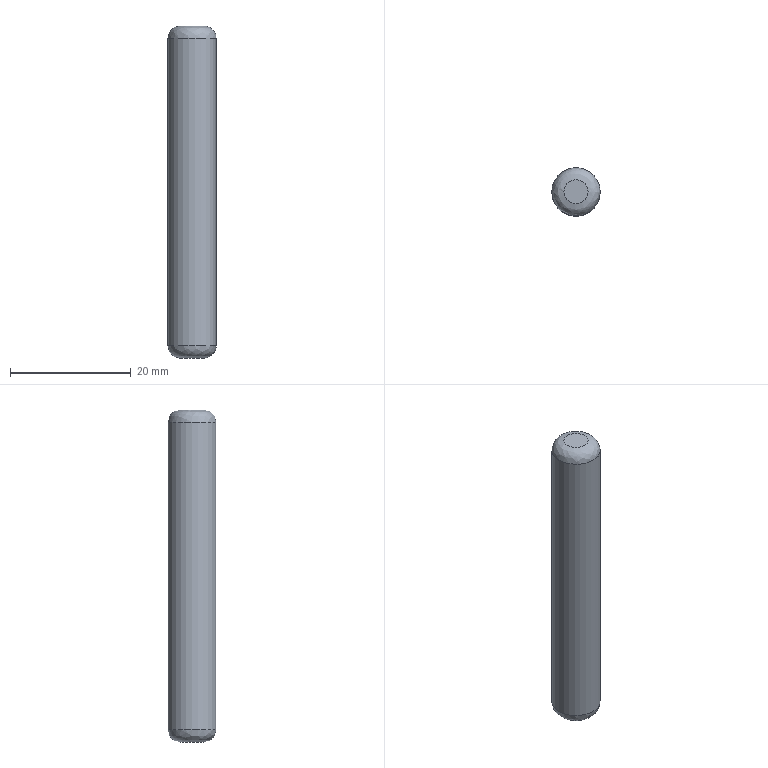Part | STEP file | 1 solid | 5 faces | box 8 x 8 x 55 mm | volume 2726 mm3 | plane 2 | spline 2 | cylinder 1 | commonest cylinder face diameters 8 x1
STEP:
#1=CARTESIAN_POINT('',(0.,0.,0.));
#2=DIRECTION('',(0.,0.,1.));
#3=DIRECTION('',(1.,0.,0.));
#4=AXIS2_PLACEMENT_3D('',#1,#2,#3);
#5=CARTESIAN_POINT('',(1516.247,357.48,61.619));
#6=VERTEX_POINT('',#5);
#7=CARTESIAN_POINT('',(1512.247,357.48,61.619));
#8=DIRECTION('',(0.,0.,-1.));
#9=DIRECTION('',(1.,0.,0.));
#10=AXIS2_PLACEMENT_3D('',#7,#8,#9);
#11=CIRCLE('',#10,4.);
#12=CARTESIAN_POINT('',(1512.247,357.48,8.619));
#13=DIRECTION('',(0.,0.,1.));
#14=DIRECTION('',(1.,0.,0.));
#15=AXIS2_PLACEMENT_3D('',#12,#13,#14);
#16=CYLINDRICAL_SURFACE('',#15,4.);
#17=CARTESIAN_POINT('',(6.283,53.));
#18=DIRECTION('',(-1.,0.));
#19=VECTOR('',#18,1.);
#20=LINE('',#17,#19);
#21=(GEOMETRIC_REPRESENTATION_CONTEXT(2)PARAMETRIC_REPRESENTATION_CONTEXT()REPRESENTATION_CONTEXT('',''));
#22=DEFINITIONAL_REPRESENTATION('',(#20),#21);
#23=PCURVE('',#16,#22);
#24=CARTESIAN_POINT('',(1508.247,357.48,61.619));
#25=CARTESIAN_POINT('',(1508.247,365.48,61.619));
#26=CARTESIAN_POINT('',(1516.247,365.48,61.619));
#27=CARTESIAN_POINT('',(1516.247,357.48,61.619));
#28=CARTESIAN_POINT('',(1516.247,349.48,61.619));
#29=CARTESIAN_POINT('',(1508.247,349.48,61.619));
#30=CARTESIAN_POINT('',(1508.247,357.48,61.619));
#31=CARTESIAN_POINT('',(1508.247,357.48,62.791));
#32=CARTESIAN_POINT('',(1508.247,365.48,62.791));
#33=CARTESIAN_POINT('',(1516.247,365.48,62.791));
#34=CARTESIAN_POINT('',(1516.247,357.48,62.791));
#35=CARTESIAN_POINT('',(1516.247,349.48,62.791));
#36=CARTESIAN_POINT('',(1508.247,349.48,62.791));
#37=CARTESIAN_POINT('',(1508.247,357.48,62.791));
#38=CARTESIAN_POINT('',(1509.076,357.48,63.619));
#39=CARTESIAN_POINT('',(1509.076,363.824,63.619));
#40=CARTESIAN_POINT('',(1515.419,363.824,63.619));
#41=CARTESIAN_POINT('',(1515.419,357.48,63.619));
#42=CARTESIAN_POINT('',(1515.419,351.137,63.619));
#43=CARTESIAN_POINT('',(1509.076,351.137,63.619));
#44=CARTESIAN_POINT('',(1509.076,357.48,63.619));
#45=CARTESIAN_POINT('',(1510.247,357.48,63.619));
#46=CARTESIAN_POINT('',(1510.247,361.48,63.619));
#47=CARTESIAN_POINT('',(1514.247,361.48,63.619));
#48=CARTESIAN_POINT('',(1514.247,357.48,63.619));
#49=CARTESIAN_POINT('',(1514.247,353.48,63.619));
#50=CARTESIAN_POINT('',(1510.247,353.48,63.619));
#51=CARTESIAN_POINT('',(1510.247,357.48,63.619));
#52=(BOUNDED_SURFACE()B_SPLINE_SURFACE(3,3,((#24,#25,#26,#27,#28,#29,#30),(#31,#32,#33,#34,#35,#36,#37),(#38,#39,#40,#41,#42,#43,#44),(#45,#46,#47,#48,#49,#50,#51)),.UNSPECIFIED.,.F.,.T.,.F.)B_SPLINE_SURFACE_WITH_KNOTS((4,4),(1,3,3,3,1),(0.,1.),(-0.5,0.,0.5,1.,1.5),.UNSPECIFIED.)GEOMETRIC_REPRESENTATION_ITEM()RATIONAL_B_SPLINE_SURFACE(((1.,0.3333,0.3333,1.,0.3333,0.3333,1.),(0.8047,0.2682,0.2682,0.8047,0.2682,0.2682,0.8047),(0.8047,0.2682,0.2682,0.8047,0.2682,0.2682,0.8047),(1.,0.3333,0.3333,1.,0.3333,0.3333,1.)))REPRESENTATION_ITEM('')SURFACE());
#53=CARTESIAN_POINT('',(0.,0.5));
#54=CARTESIAN_POINT('',(0.,0.5235));
#55=CARTESIAN_POINT('',(0.,0.5649));
#56=CARTESIAN_POINT('',(0.,0.6146));
#57=CARTESIAN_POINT('',(0.,0.6575));
#58=CARTESIAN_POINT('',(0.,0.696));
#59=CARTESIAN_POINT('',(0.,0.7322));
#60=CARTESIAN_POINT('',(0.,0.7678));
#61=CARTESIAN_POINT('',(0.,0.804));
#62=CARTESIAN_POINT('',(0.,0.8425));
#63=CARTESIAN_POINT('',(0.,0.8856));
#64=CARTESIAN_POINT('',(0.,0.9343));
#65=CARTESIAN_POINT('',(0.,1.));
#66=CARTESIAN_POINT('',(0.,1.066));
#67=CARTESIAN_POINT('',(0.,1.114));
#68=CARTESIAN_POINT('',(0.,1.158));
#69=CARTESIAN_POINT('',(0.,1.196));
#70=CARTESIAN_POINT('',(0.,1.232));
#71=CARTESIAN_POINT('',(0.,1.268));
#72=CARTESIAN_POINT('',(0.,1.304));
#73=CARTESIAN_POINT('',(0.,1.343));
#74=CARTESIAN_POINT('',(0.,1.385));
#75=CARTESIAN_POINT('',(0.,1.435));
#76=CARTESIAN_POINT('',(0.,1.476));
#77=CARTESIAN_POINT('',(0.,1.5));
#78=B_SPLINE_CURVE_WITH_KNOTS('',3,(#53,#54,#55,#56,#57,#58,#59,#60,#61,#62,#63,#64,#65,#66,#67,#68,#69,#70,#71,#72,#73,#74,#75,#76,#77),.UNSPECIFIED.,.F.,.F.,(4,1,1,1,1,1,1,1,1,1,1,1,1,1,1,1,1,1,1,1,1,1,4),(0.,0.2856,0.5712,0.8568,1.142,1.428,1.714,1.999,2.285,2.57,2.856,3.142,3.427,3.713,3.998,4.284,4.57,4.855,5.141,5.426,5.712,5.998,6.283),.QUASI_UNIFORM_KNOTS.);
#79=(GEOMETRIC_REPRESENTATION_CONTEXT(2)PARAMETRIC_REPRESENTATION_CONTEXT()REPRESENTATION_CONTEXT('',''));
#80=DEFINITIONAL_REPRESENTATION('',(#78),#79);
#81=PCURVE('',#52,#80);
#82=SURFACE_CURVE('',#11,(#23,#81),.PCURVE_S1.);
#83=EDGE_CURVE('',#6,#6,#82,.T.);
#84=ORIENTED_EDGE('',*,*,#83,.T.);
#85=CARTESIAN_POINT('',(1516.247,357.48,10.619));
#86=VERTEX_POINT('',#85);
#87=CARTESIAN_POINT('',(1516.247,357.48,10.619));
#88=CARTESIAN_POINT('',(1516.247,357.48,61.619));
#89=B_SPLINE_CURVE_WITH_KNOTS('',1,(#87,#88),.UNSPECIFIED.,.F.,.F.,(2,2),(2.,53.),.PIECEWISE_BEZIER_KNOTS.);
#90=CARTESIAN_POINT('',(0.,0.));
#91=DIRECTION('',(0.,1.));
#92=VECTOR('',#91,1.);
#93=LINE('',#90,#92);
#94=(GEOMETRIC_REPRESENTATION_CONTEXT(2)PARAMETRIC_REPRESENTATION_CONTEXT()REPRESENTATION_CONTEXT('',''));
#95=DEFINITIONAL_REPRESENTATION('',(#93),#94);
#96=PCURVE('',#16,#95);
#97=CARTESIAN_POINT('',(6.283,0.));
#98=DIRECTION('',(0.,1.));
#99=VECTOR('',#98,1.);
#100=LINE('',#97,#99);
#101=(GEOMETRIC_REPRESENTATION_CONTEXT(2)PARAMETRIC_REPRESENTATION_CONTEXT()REPRESENTATION_CONTEXT('',''));
#102=DEFINITIONAL_REPRESENTATION('',(#100),#101);
#103=PCURVE('',#16,#102);
#104=SEAM_CURVE('',#89,(#96,#103),.PCURVE_S1.);
#105=EDGE_CURVE('',#86,#6,#104,.T.);
#106=ORIENTED_EDGE('',*,*,#105,.F.);
#107=CARTESIAN_POINT('',(1512.247,357.48,10.619));
#108=DIRECTION('',(0.,0.,1.));
#109=DIRECTION('',(1.,0.,0.));
#110=AXIS2_PLACEMENT_3D('',#107,#108,#109);
#111=CIRCLE('',#110,4.);
#112=CARTESIAN_POINT('',(0.,2.));
#113=DIRECTION('',(1.,0.));
#114=VECTOR('',#113,1.);
#115=LINE('',#112,#114);
#116=(GEOMETRIC_REPRESENTATION_CONTEXT(2)PARAMETRIC_REPRESENTATION_CONTEXT()REPRESENTATION_CONTEXT('',''));
#117=DEFINITIONAL_REPRESENTATION('',(#115),#116);
#118=PCURVE('',#16,#117);
#119=CARTESIAN_POINT('',(1510.247,357.48,8.619));
#120=CARTESIAN_POINT('',(1510.247,361.48,8.619));
#121=CARTESIAN_POINT('',(1514.247,361.48,8.619));
#122=CARTESIAN_POINT('',(1514.247,357.48,8.619));
#123=CARTESIAN_POINT('',(1514.247,353.48,8.619));
#124=CARTESIAN_POINT('',(1510.247,353.48,8.619));
#125=CARTESIAN_POINT('',(1510.247,357.48,8.619));
#126=CARTESIAN_POINT('',(1509.076,357.48,8.619));
#127=CARTESIAN_POINT('',(1509.076,363.824,8.619));
#128=CARTESIAN_POINT('',(1515.419,363.824,8.619));
#129=CARTESIAN_POINT('',(1515.419,357.48,8.619));
#130=CARTESIAN_POINT('',(1515.419,351.137,8.619));
#131=CARTESIAN_POINT('',(1509.076,351.137,8.619));
#132=CARTESIAN_POINT('',(1509.076,357.48,8.619));
#133=CARTESIAN_POINT('',(1508.247,357.48,9.447));
#134=CARTESIAN_POINT('',(1508.247,365.48,9.447));
#135=CARTESIAN_POINT('',(1516.247,365.48,9.447));
#136=CARTESIAN_POINT('',(1516.247,357.48,9.447));
#137=CARTESIAN_POINT('',(1516.247,349.48,9.447));
#138=CARTESIAN_POINT('',(1508.247,349.48,9.447));
#139=CARTESIAN_POINT('',(1508.247,357.48,9.447));
#140=CARTESIAN_POINT('',(1508.247,357.48,10.619));
#141=CARTESIAN_POINT('',(1508.247,365.48,10.619));
#142=CARTESIAN_POINT('',(1516.247,365.48,10.619));
#143=CARTESIAN_POINT('',(1516.247,357.48,10.619));
#144=CARTESIAN_POINT('',(1516.247,349.48,10.619));
#145=CARTESIAN_POINT('',(1508.247,349.48,10.619));
#146=CARTESIAN_POINT('',(1508.247,357.48,10.619));
#147=(BOUNDED_SURFACE()B_SPLINE_SURFACE(3,3,((#119,#120,#121,#122,#123,#124,#125),(#126,#127,#128,#129,#130,#131,#132),(#133,#134,#135,#136,#137,#138,#139),(#140,#141,#142,#143,#144,#145,#146)),.UNSPECIFIED.,.F.,.T.,.F.)B_SPLINE_SURFACE_WITH_KNOTS((4,4),(1,3,3,3,1),(0.,1.),(-0.5,0.,0.5,1.,1.5),.UNSPECIFIED.)GEOMETRIC_REPRESENTATION_ITEM()RATIONAL_B_SPLINE_SURFACE(((1.,0.3333,0.3333,1.,0.3333,0.3333,1.),(0.8047,0.2682,0.2682,0.8047,0.2682,0.2682,0.8047),(0.8047,0.2682,0.2682,0.8047,0.2682,0.2682,0.8047),(1.,0.3333,0.3333,1.,0.3333,0.3333,1.)))REPRESENTATION_ITEM('')SURFACE());
#148=CARTESIAN_POINT('',(1.,1.5));
#149=CARTESIAN_POINT('',(1.,1.476));
#150=CARTESIAN_POINT('',(1.,1.435));
#151=CARTESIAN_POINT('',(1.,1.385));
#152=CARTESIAN_POINT('',(1.,1.343));
#153=CARTESIAN_POINT('',(1.,1.304));
#154=CARTESIAN_POINT('',(1.,1.268));
#155=CARTESIAN_POINT('',(1.,1.232));
#156=CARTESIAN_POINT('',(1.,1.196));
#157=CARTESIAN_POINT('',(1.,1.158));
#158=CARTESIAN_POINT('',(1.,1.114));
#159=CARTESIAN_POINT('',(1.,1.066));
#160=CARTESIAN_POINT('',(1.,1.));
#161=CARTESIAN_POINT('',(1.,0.9343));
#162=CARTESIAN_POINT('',(1.,0.8856));
#163=CARTESIAN_POINT('',(1.,0.8425));
#164=CARTESIAN_POINT('',(1.,0.804));
#165=CARTESIAN_POINT('',(1.,0.7678));
#166=CARTESIAN_POINT('',(1.,0.7322));
#167=CARTESIAN_POINT('',(1.,0.696));
#168=CARTESIAN_POINT('',(1.,0.6575));
#169=CARTESIAN_POINT('',(1.,0.6146));
#170=CARTESIAN_POINT('',(1.,0.5649));
#171=CARTESIAN_POINT('',(1.,0.5235));
#172=CARTESIAN_POINT('',(1.,0.5));
#173=B_SPLINE_CURVE_WITH_KNOTS('',3,(#148,#149,#150,#151,#152,#153,#154,#155,#156,#157,#158,#159,#160,#161,#162,#163,#164,#165,#166,#167,#168,#169,#170,#171,#172),.UNSPECIFIED.,.F.,.F.,(4,1,1,1,1,1,1,1,1,1,1,1,1,1,1,1,1,1,1,1,1,1,4),(0.,0.2856,0.5712,0.8568,1.142,1.428,1.714,1.999,2.285,2.57,2.856,3.142,3.427,3.713,3.998,4.284,4.57,4.855,5.141,5.426,5.712,5.998,6.283),.QUASI_UNIFORM_KNOTS.);
#174=(GEOMETRIC_REPRESENTATION_CONTEXT(2)PARAMETRIC_REPRESENTATION_CONTEXT()REPRESENTATION_CONTEXT('',''));
#175=DEFINITIONAL_REPRESENTATION('',(#173),#174);
#176=PCURVE('',#147,#175);
#177=SURFACE_CURVE('',#111,(#118,#176),.PCURVE_S1.);
#178=EDGE_CURVE('',#86,#86,#177,.T.);
#179=ORIENTED_EDGE('',*,*,#178,.T.);
#180=ORIENTED_EDGE('',*,*,#105,.T.);
#181=EDGE_LOOP('',(#84,#106,#179,#180));
#182=FACE_BOUND('',#181,.T.);
#183=ADVANCED_FACE('',(#182),#16,.T.);
#184=CARTESIAN_POINT('',(1514.247,357.48,8.619));
#185=VERTEX_POINT('',#184);
#186=CARTESIAN_POINT('',(1512.247,357.48,8.619));
#187=DIRECTION('',(0.,0.,-1.));
#188=DIRECTION('',(1.,0.,0.));
#189=AXIS2_PLACEMENT_3D('',#186,#187,#188);
#190=CIRCLE('',#189,2.);
#191=CARTESIAN_POINT('',(1512.247,357.48,8.619));
#192=DIRECTION('',(0.,0.,-1.));
#193=DIRECTION('',(-1.,0.,0.));
#194=AXIS2_PLACEMENT_3D('',#191,#192,#193);
#195=PLANE('',#194);
#196=CARTESIAN_POINT('',(0.,0.));
#197=DIRECTION('',(-1.,0.));
#198=AXIS2_PLACEMENT_2D('',#196,#197);
#199=CIRCLE('',#198,2.);
#200=(GEOMETRIC_REPRESENTATION_CONTEXT(2)PARAMETRIC_REPRESENTATION_CONTEXT()REPRESENTATION_CONTEXT('',''));
#201=DEFINITIONAL_REPRESENTATION('',(#199),#200);
#202=PCURVE('',#195,#201);
#203=CARTESIAN_POINT('',(0.,0.5));
#204=CARTESIAN_POINT('',(0.,0.5235));
#205=CARTESIAN_POINT('',(0.,0.5649));
#206=CARTESIAN_POINT('',(0.,0.6146));
#207=CARTESIAN_POINT('',(0.,0.6575));
#208=CARTESIAN_POINT('',(0.,0.696));
#209=CARTESIAN_POINT('',(0.,0.7322));
#210=CARTESIAN_POINT('',(0.,0.7678));
#211=CARTESIAN_POINT('',(0.,0.804));
#212=CARTESIAN_POINT('',(0.,0.8425));
#213=CARTESIAN_POINT('',(0.,0.8856));
#214=CARTESIAN_POINT('',(0.,0.9343));
#215=CARTESIAN_POINT('',(0.,1.));
#216=CARTESIAN_POINT('',(0.,1.066));
#217=CARTESIAN_POINT('',(0.,1.114));
#218=CARTESIAN_POINT('',(0.,1.158));
#219=CARTESIAN_POINT('',(0.,1.196));
#220=CARTESIAN_POINT('',(0.,1.232));
#221=CARTESIAN_POINT('',(0.,1.268));
#222=CARTESIAN_POINT('',(0.,1.304));
#223=CARTESIAN_POINT('',(0.,1.343));
#224=CARTESIAN_POINT('',(0.,1.385));
#225=CARTESIAN_POINT('',(0.,1.435));
#226=CARTESIAN_POINT('',(0.,1.476));
#227=CARTESIAN_POINT('',(0.,1.5));
#228=B_SPLINE_CURVE_WITH_KNOTS('',3,(#203,#204,#205,#206,#207,#208,#209,#210,#211,#212,#213,#214,#215,#216,#217,#218,#219,#220,#221,#222,#223,#224,#225,#226,#227),.UNSPECIFIED.,.F.,.F.,(4,1,1,1,1,1,1,1,1,1,1,1,1,1,1,1,1,1,1,1,1,1,4),(0.,0.2856,0.5712,0.8568,1.142,1.428,1.714,1.999,2.285,2.57,2.856,3.142,3.427,3.713,3.998,4.284,4.57,4.855,5.141,5.426,5.712,5.998,6.283),.QUASI_UNIFORM_KNOTS.);
#229=(GEOMETRIC_REPRESENTATION_CONTEXT(2)PARAMETRIC_REPRESENTATION_CONTEXT()REPRESENTATION_CONTEXT('',''));
#230=DEFINITIONAL_REPRESENTATION('',(#228),#229);
#231=PCURVE('',#147,#230);
#232=SURFACE_CURVE('',#190,(#202,#231),.PCURVE_S1.);
#233=EDGE_CURVE('',#185,#185,#232,.T.);
#234=ORIENTED_EDGE('',*,*,#233,.T.);
#235=EDGE_LOOP('',(#234));
#236=FACE_BOUND('',#235,.T.);
#237=ADVANCED_FACE('',(#236),#195,.T.);
#238=CARTESIAN_POINT('',(1514.247,357.48,63.619));
#239=VERTEX_POINT('',#238);
#240=CARTESIAN_POINT('',(1512.247,357.48,63.619));
#241=DIRECTION('',(0.,0.,1.));
#242=DIRECTION('',(1.,0.,0.));
#243=AXIS2_PLACEMENT_3D('',#240,#241,#242);
#244=CIRCLE('',#243,2.);
#245=CARTESIAN_POINT('',(1512.247,357.48,63.619));
#246=DIRECTION('',(0.,0.,-1.));
#247=DIRECTION('',(-1.,0.,0.));
#248=AXIS2_PLACEMENT_3D('',#245,#246,#247);
#249=PLANE('',#248);
#250=CARTESIAN_POINT('',(-2.,0.));
#251=CARTESIAN_POINT('',(-2.,3.464));
#252=CARTESIAN_POINT('',(1.,1.732));
#253=CARTESIAN_POINT('',(4.,0.));
#254=CARTESIAN_POINT('',(1.,-1.732));
#255=CARTESIAN_POINT('',(-2.,-3.464));
#256=CARTESIAN_POINT('',(-2.,0.));
#257=(BOUNDED_CURVE()B_SPLINE_CURVE(2,(#250,#251,#252,#253,#254,#255,#256),.UNSPECIFIED.,.T.,.F.)B_SPLINE_CURVE_WITH_KNOTS((1,2,2,2,2,1),(-2.094,0.,2.094,4.189,6.283,8.378),.UNSPECIFIED.)CURVE()GEOMETRIC_REPRESENTATION_ITEM()RATIONAL_B_SPLINE_CURVE((1.,0.5,1.,0.5,1.,0.5,1.))REPRESENTATION_ITEM(''));
#258=(GEOMETRIC_REPRESENTATION_CONTEXT(2)PARAMETRIC_REPRESENTATION_CONTEXT()REPRESENTATION_CONTEXT('',''));
#259=DEFINITIONAL_REPRESENTATION('',(#257),#258);
#260=PCURVE('',#249,#259);
#261=CARTESIAN_POINT('',(1.,1.5));
#262=CARTESIAN_POINT('',(1.,1.476));
#263=CARTESIAN_POINT('',(1.,1.435));
#264=CARTESIAN_POINT('',(1.,1.385));
#265=CARTESIAN_POINT('',(1.,1.343));
#266=CARTESIAN_POINT('',(1.,1.304));
#267=CARTESIAN_POINT('',(1.,1.268));
#268=CARTESIAN_POINT('',(1.,1.232));
#269=CARTESIAN_POINT('',(1.,1.196));
#270=CARTESIAN_POINT('',(1.,1.158));
#271=CARTESIAN_POINT('',(1.,1.114));
#272=CARTESIAN_POINT('',(1.,1.066));
#273=CARTESIAN_POINT('',(1.,1.));
#274=CARTESIAN_POINT('',(1.,0.9343));
#275=CARTESIAN_POINT('',(1.,0.8856));
#276=CARTESIAN_POINT('',(1.,0.8425));
#277=CARTESIAN_POINT('',(1.,0.804));
#278=CARTESIAN_POINT('',(1.,0.7678));
#279=CARTESIAN_POINT('',(1.,0.7322));
#280=CARTESIAN_POINT('',(1.,0.696));
#281=CARTESIAN_POINT('',(1.,0.6575));
#282=CARTESIAN_POINT('',(1.,0.6146));
#283=CARTESIAN_POINT('',(1.,0.5649));
#284=CARTESIAN_POINT('',(1.,0.5235));
#285=CARTESIAN_POINT('',(1.,0.5));
#286=B_SPLINE_CURVE_WITH_KNOTS('',3,(#261,#262,#263,#264,#265,#266,#267,#268,#269,#270,#271,#272,#273,#274,#275,#276,#277,#278,#279,#280,#281,#282,#283,#284,#285),.UNSPECIFIED.,.F.,.F.,(4,1,1,1,1,1,1,1,1,1,1,1,1,1,1,1,1,1,1,1,1,1,4),(0.,0.2856,0.5712,0.8568,1.142,1.428,1.714,1.999,2.285,2.57,2.856,3.142,3.427,3.713,3.998,4.284,4.57,4.855,5.141,5.426,5.712,5.998,6.283),.QUASI_UNIFORM_KNOTS.);
#287=(GEOMETRIC_REPRESENTATION_CONTEXT(2)PARAMETRIC_REPRESENTATION_CONTEXT()REPRESENTATION_CONTEXT('',''));
#288=DEFINITIONAL_REPRESENTATION('',(#286),#287);
#289=PCURVE('',#52,#288);
#290=SURFACE_CURVE('',#244,(#260,#289),.PCURVE_S1.);
#291=EDGE_CURVE('',#239,#239,#290,.T.);
#292=ORIENTED_EDGE('',*,*,#291,.T.);
#293=EDGE_LOOP('',(#292));
#294=FACE_BOUND('',#293,.T.);
#295=ADVANCED_FACE('',(#294),#249,.F.);
#296=ORIENTED_EDGE('',*,*,#291,.F.);
#297=CARTESIAN_POINT('',(1516.247,357.48,61.619));
#298=CARTESIAN_POINT('',(1516.247,357.48,62.791));
#299=CARTESIAN_POINT('',(1515.419,357.48,63.619));
#300=CARTESIAN_POINT('',(1514.247,357.48,63.619));
#301=(BOUNDED_CURVE()B_SPLINE_CURVE(3,(#297,#298,#299,#300),.UNSPECIFIED.,.F.,.F.)B_SPLINE_CURVE_WITH_KNOTS((4,4),(0.,1.),.PIECEWISE_BEZIER_KNOTS.)CURVE()GEOMETRIC_REPRESENTATION_ITEM()RATIONAL_B_SPLINE_CURVE((1.,0.8047,0.8047,1.))REPRESENTATION_ITEM(''));
#302=CARTESIAN_POINT('',(0.,1.5));
#303=DIRECTION('',(1.,0.));
#304=VECTOR('',#303,1.);
#305=LINE('',#302,#304);
#306=(GEOMETRIC_REPRESENTATION_CONTEXT(2)PARAMETRIC_REPRESENTATION_CONTEXT()REPRESENTATION_CONTEXT('',''));
#307=DEFINITIONAL_REPRESENTATION('',(#305),#306);
#308=PCURVE('',#52,#307);
#309=CARTESIAN_POINT('',(0.,0.5));
#310=DIRECTION('',(1.,0.));
#311=VECTOR('',#310,1.);
#312=LINE('',#309,#311);
#313=(GEOMETRIC_REPRESENTATION_CONTEXT(2)PARAMETRIC_REPRESENTATION_CONTEXT()REPRESENTATION_CONTEXT('',''));
#314=DEFINITIONAL_REPRESENTATION('',(#312),#313);
#315=PCURVE('',#52,#314);
#316=SEAM_CURVE('',#301,(#308,#315),.PCURVE_S1.);
#317=EDGE_CURVE('',#6,#239,#316,.T.);
#318=ORIENTED_EDGE('',*,*,#317,.F.);
#319=ORIENTED_EDGE('',*,*,#83,.F.);
#320=ORIENTED_EDGE('',*,*,#317,.T.);
#321=EDGE_LOOP('',(#296,#318,#319,#320));
#322=FACE_BOUND('',#321,.T.);
#323=ADVANCED_FACE('',(#322),#52,.T.);
#324=ORIENTED_EDGE('',*,*,#178,.F.);
#325=CARTESIAN_POINT('',(1514.247,357.48,8.619));
#326=CARTESIAN_POINT('',(1515.419,357.48,8.619));
#327=CARTESIAN_POINT('',(1516.247,357.48,9.447));
#328=CARTESIAN_POINT('',(1516.247,357.48,10.619));
#329=(BOUNDED_CURVE()B_SPLINE_CURVE(3,(#325,#326,#327,#328),.UNSPECIFIED.,.F.,.F.)B_SPLINE_CURVE_WITH_KNOTS((4,4),(0.,1.),.PIECEWISE_BEZIER_KNOTS.)CURVE()GEOMETRIC_REPRESENTATION_ITEM()RATIONAL_B_SPLINE_CURVE((1.,0.8047,0.8047,1.))REPRESENTATION_ITEM(''));
#330=CARTESIAN_POINT('',(0.,1.5));
#331=DIRECTION('',(1.,0.));
#332=VECTOR('',#331,1.);
#333=LINE('',#330,#332);
#334=(GEOMETRIC_REPRESENTATION_CONTEXT(2)PARAMETRIC_REPRESENTATION_CONTEXT()REPRESENTATION_CONTEXT('',''));
#335=DEFINITIONAL_REPRESENTATION('',(#333),#334);
#336=PCURVE('',#147,#335);
#337=CARTESIAN_POINT('',(0.,0.5));
#338=DIRECTION('',(1.,0.));
#339=VECTOR('',#338,1.);
#340=LINE('',#337,#339);
#341=(GEOMETRIC_REPRESENTATION_CONTEXT(2)PARAMETRIC_REPRESENTATION_CONTEXT()REPRESENTATION_CONTEXT('',''));
#342=DEFINITIONAL_REPRESENTATION('',(#340),#341);
#343=PCURVE('',#147,#342);
#344=SEAM_CURVE('',#329,(#336,#343),.PCURVE_S1.);
#345=EDGE_CURVE('',#185,#86,#344,.T.);
#346=ORIENTED_EDGE('',*,*,#345,.F.);
#347=ORIENTED_EDGE('',*,*,#233,.F.);
#348=ORIENTED_EDGE('',*,*,#345,.T.);
#349=EDGE_LOOP('',(#324,#346,#347,#348));
#350=FACE_BOUND('',#349,.T.);
#351=ADVANCED_FACE('',(#350),#147,.T.);
#352=CLOSED_SHELL('',(#183,#237,#295,#323,#351));
#353=MANIFOLD_SOLID_BREP('',#352);
#354=(LENGTH_UNIT()NAMED_UNIT(*)SI_UNIT(.MILLI.,.METRE.));
#355=UNCERTAINTY_MEASURE_WITH_UNIT(LENGTH_MEASURE(0.00001),#354,'','');
#356=(NAMED_UNIT(*)PLANE_ANGLE_UNIT()SI_UNIT($,.RADIAN.));
#357=(NAMED_UNIT(*)SI_UNIT($,.STERADIAN.)SOLID_ANGLE_UNIT());
#358=(GEOMETRIC_REPRESENTATION_CONTEXT(3)GLOBAL_UNCERTAINTY_ASSIGNED_CONTEXT((#355))GLOBAL_UNIT_ASSIGNED_CONTEXT((#354,#356,#357))REPRESENTATION_CONTEXT('',''));
#359=ADVANCED_BREP_SHAPE_REPRESENTATION('',(#4,#353),#358);